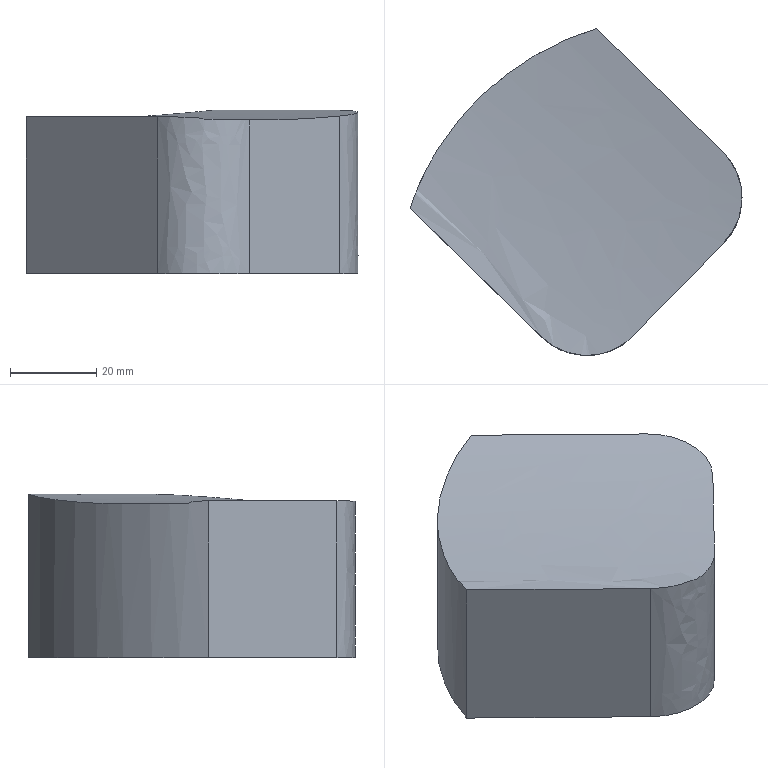Part | NX | features solid 2 | 1 solid | 10 faces | box 76.93 x 75.708 x 37.827 mm | volume 128623 mm3 | spline 6 | plane 2 | cylinder 1 | cone 1 | commonest cylinder face diameters 10 x1
STEP:
#1=CARTESIAN_POINT('',(-596.108,399.175,9.827));
#2=VERTEX_POINT('',#1);
#3=CARTESIAN_POINT('',(-566.89,370.687,9.827));
#4=VERTEX_POINT('',#3);
#5=CARTESIAN_POINT('',(-566.89,370.687,9.827));
#6=CARTESIAN_POINT('',(-576.63,380.183,9.827));
#7=CARTESIAN_POINT('',(-586.369,389.679,9.827));
#8=CARTESIAN_POINT('',(-596.108,399.175,9.827));
#9=B_SPLINE_CURVE_WITH_KNOTS('',3,(#5,#6,#7,#8),.UNSPECIFIED.,.F.,.F.,(4,4),(0.04669,0.0875),.UNSPECIFIED.);
#10=EDGE_CURVE('',#2,#4,#9,.F.);
#11=ORIENTED_EDGE('',*,*,#10,.T.);
#12=CARTESIAN_POINT('',(-566.89,370.687,-28.));
#13=VERTEX_POINT('',#12);
#14=CARTESIAN_POINT('',(-566.89,370.687,9.827));
#15=CARTESIAN_POINT('',(-566.89,370.687,-2.782));
#16=CARTESIAN_POINT('',(-566.89,370.687,-15.391));
#17=CARTESIAN_POINT('',(-566.89,370.687,-28.));
#18=B_SPLINE_CURVE_WITH_KNOTS('',3,(#14,#15,#16,#17),.UNSPECIFIED.,.F.,.F.,(4,4),(0.,0.03783),.UNSPECIFIED.);
#19=EDGE_CURVE('',#4,#13,#18,.T.);
#20=ORIENTED_EDGE('',*,*,#19,.T.);
#21=CARTESIAN_POINT('',(-596.108,399.175,-28.));
#22=VERTEX_POINT('',#21);
#23=CARTESIAN_POINT('',(-596.108,399.175,-28.));
#24=CARTESIAN_POINT('',(-586.369,389.679,-28.));
#25=CARTESIAN_POINT('',(-576.63,380.183,-28.));
#26=CARTESIAN_POINT('',(-566.89,370.687,-28.));
#27=B_SPLINE_CURVE_WITH_KNOTS('',3,(#23,#24,#25,#26),.UNSPECIFIED.,.F.,.F.,(4,4),(0.,1.),.UNSPECIFIED.);
#28=EDGE_CURVE('',#22,#13,#27,.T.);
#29=ORIENTED_EDGE('',*,*,#28,.F.);
#30=CARTESIAN_POINT('',(-596.108,399.175,-28.));
#31=CARTESIAN_POINT('',(-596.108,399.175,-15.391));
#32=CARTESIAN_POINT('',(-596.108,399.175,-2.782));
#33=CARTESIAN_POINT('',(-596.108,399.175,9.827));
#34=B_SPLINE_CURVE_WITH_KNOTS('',3,(#30,#31,#32,#33),.UNSPECIFIED.,.F.,.F.,(4,4),(0.164,0.2018),.UNSPECIFIED.);
#35=EDGE_CURVE('',#22,#2,#34,.T.);
#36=ORIENTED_EDGE('',*,*,#35,.T.);
#37=EDGE_LOOP('',(#11,#20,#29,#36));
#38=FACE_BOUND('',#37,.T.);
#39=CARTESIAN_POINT('',(-566.89,370.687,9.827));
#40=CARTESIAN_POINT('',(-576.63,380.183,9.827));
#41=CARTESIAN_POINT('',(-586.369,389.679,9.827));
#42=CARTESIAN_POINT('',(-596.108,399.175,9.827));
#43=CARTESIAN_POINT('',(-566.89,370.687,-2.782));
#44=CARTESIAN_POINT('',(-576.63,380.183,-2.782));
#45=CARTESIAN_POINT('',(-586.369,389.679,-2.782));
#46=CARTESIAN_POINT('',(-596.108,399.175,-2.782));
#47=CARTESIAN_POINT('',(-566.89,370.687,-15.391));
#48=CARTESIAN_POINT('',(-576.63,380.183,-15.391));
#49=CARTESIAN_POINT('',(-586.369,389.679,-15.391));
#50=CARTESIAN_POINT('',(-596.108,399.175,-15.391));
#51=CARTESIAN_POINT('',(-566.89,370.687,-28.));
#52=CARTESIAN_POINT('',(-576.63,380.183,-28.));
#53=CARTESIAN_POINT('',(-586.369,389.679,-28.));
#54=CARTESIAN_POINT('',(-596.108,399.175,-28.));
#55=B_SPLINE_SURFACE_WITH_KNOTS('',3,3,((#39,#40,#41,#42),(#43,#44,#45,#46),(#47,#48,#49,#50),(#51,#52,#53,#54)),.UNSPECIFIED.,.F.,.F.,.F.,(4,4),(4,4),(0.2675,0.6667),(0.57,0.7724),.UNSPECIFIED.);
#56=ADVANCED_FACE('',(#38),#55,.T.);
#57=CARTESIAN_POINT('',(-639.292,357.48,-28.));
#58=VERTEX_POINT('',#57);
#59=CARTESIAN_POINT('',(-608.776,327.727,-28.));
#60=VERTEX_POINT('',#59);
#61=CARTESIAN_POINT('',(-608.776,327.727,-28.));
#62=CARTESIAN_POINT('',(-618.948,337.645,-28.));
#63=CARTESIAN_POINT('',(-629.12,347.562,-28.));
#64=CARTESIAN_POINT('',(-639.292,357.48,-28.));
#65=B_SPLINE_CURVE_WITH_KNOTS('',3,(#61,#62,#63,#64),.UNSPECIFIED.,.F.,.F.,(4,4),(0.,1.),.UNSPECIFIED.);
#66=EDGE_CURVE('',#58,#60,#65,.F.);
#67=ORIENTED_EDGE('',*,*,#66,.T.);
#68=CARTESIAN_POINT('',(-608.776,327.727,8.344));
#69=VERTEX_POINT('',#68);
#70=CARTESIAN_POINT('',(-608.776,327.727,-28.));
#71=CARTESIAN_POINT('',(-608.776,327.727,-15.885));
#72=CARTESIAN_POINT('',(-608.776,327.727,-3.77));
#73=CARTESIAN_POINT('',(-608.776,327.727,8.344));
#74=B_SPLINE_CURVE_WITH_KNOTS('',3,(#70,#71,#72,#73),.UNSPECIFIED.,.F.,.F.,(4,4),(0.,0.03634),.UNSPECIFIED.);
#75=EDGE_CURVE('',#60,#69,#74,.T.);
#76=ORIENTED_EDGE('',*,*,#75,.T.);
#77=CARTESIAN_POINT('',(-639.292,357.48,8.344));
#78=VERTEX_POINT('',#77);
#79=CARTESIAN_POINT('',(-639.292,357.48,8.344));
#80=CARTESIAN_POINT('',(-629.12,347.562,8.344));
#81=CARTESIAN_POINT('',(-618.948,337.645,8.344));
#82=CARTESIAN_POINT('',(-608.776,327.727,8.344));
#83=B_SPLINE_CURVE_WITH_KNOTS('',3,(#79,#80,#81,#82),.UNSPECIFIED.,.F.,.F.,(4,4),(0.3802,0.4229),.UNSPECIFIED.);
#84=EDGE_CURVE('',#78,#69,#83,.T.);
#85=ORIENTED_EDGE('',*,*,#84,.F.);
#86=CARTESIAN_POINT('',(-639.292,357.48,-28.));
#87=CARTESIAN_POINT('',(-639.292,357.48,-15.885));
#88=CARTESIAN_POINT('',(-639.292,357.48,-3.77));
#89=CARTESIAN_POINT('',(-639.292,357.48,8.344));
#90=B_SPLINE_CURVE_WITH_KNOTS('',3,(#86,#87,#88,#89),.UNSPECIFIED.,.F.,.F.,(4,4),(0.1647,0.2011),.UNSPECIFIED.);
#91=EDGE_CURVE('',#58,#78,#90,.T.);
#92=ORIENTED_EDGE('',*,*,#91,.F.);
#93=EDGE_LOOP('',(#67,#76,#85,#92));
#94=FACE_BOUND('',#93,.T.);
#95=CARTESIAN_POINT('',(-608.776,327.727,-28.));
#96=CARTESIAN_POINT('',(-608.776,327.727,-15.885));
#97=CARTESIAN_POINT('',(-608.776,327.727,-3.77));
#98=CARTESIAN_POINT('',(-608.776,327.727,8.344));
#99=CARTESIAN_POINT('',(-618.948,337.645,-28.));
#100=CARTESIAN_POINT('',(-618.948,337.645,-15.885));
#101=CARTESIAN_POINT('',(-618.948,337.645,-3.77));
#102=CARTESIAN_POINT('',(-618.948,337.645,8.344));
#103=CARTESIAN_POINT('',(-629.12,347.562,-28.));
#104=CARTESIAN_POINT('',(-629.12,347.562,-15.885));
#105=CARTESIAN_POINT('',(-629.12,347.562,-3.77));
#106=CARTESIAN_POINT('',(-629.12,347.562,8.344));
#107=CARTESIAN_POINT('',(-639.292,357.48,-28.));
#108=CARTESIAN_POINT('',(-639.292,357.48,-15.885));
#109=CARTESIAN_POINT('',(-639.292,357.48,-3.77));
#110=CARTESIAN_POINT('',(-639.292,357.48,8.344));
#111=B_SPLINE_SURFACE_WITH_KNOTS('',3,3,((#95,#96,#97,#98),(#99,#100,#101,#102),(#103,#104,#105,#106),(#107,#108,#109,#110)),.UNSPECIFIED.,.F.,.F.,.F.,(4,4),(4,4),(0.5587,0.76),(0.3333,0.6894),.UNSPECIFIED.);
#112=ADVANCED_FACE('',(#94),#111,.F.);
#113=ORIENTED_EDGE('',*,*,#84,.T.);
#114=CARTESIAN_POINT('',(-587.565,327.996,7.602));
#115=VERTEX_POINT('',#114);
#116=CARTESIAN_POINT('',(-608.776,327.727,8.344));
#117=CARTESIAN_POINT('',(-608.068,327.037,8.344));
#118=CARTESIAN_POINT('',(-606.545,325.819,8.337));
#119=CARTESIAN_POINT('',(-604.346,324.676,8.3));
#120=CARTESIAN_POINT('',(-602.494,324.04,8.277));
#121=CARTESIAN_POINT('',(-601.076,323.7,8.186));
#122=CARTESIAN_POINT('',(-599.594,323.499,8.343));
#123=CARTESIAN_POINT('',(-598.174,323.445,7.686));
#124=CARTESIAN_POINT('',(-596.694,323.529,7.792));
#125=CARTESIAN_POINT('',(-595.235,323.76,7.739));
#126=CARTESIAN_POINT('',(-593.792,324.137,7.712));
#127=CARTESIAN_POINT('',(-591.034,325.156,7.65));
#128=CARTESIAN_POINT('',(-588.952,326.573,7.616));
#129=CARTESIAN_POINT('',(-587.565,327.996,7.602));
#130=B_SPLINE_CURVE_WITH_KNOTS('',3,(#116,#117,#118,#119,#120,#121,#122,#123,#124,#125,#126,#127,#128,#129),.UNSPECIFIED.,.F.,.F.,(4,1,1,1,1,1,1,1,1,1,1,4),(0.,0.002926,0.005852,0.007315,0.008778,0.01024,0.0117,0.01317,0.01463,0.01609,0.01756,0.02341),.UNSPECIFIED.);
#131=EDGE_CURVE('',#69,#115,#130,.T.);
#132=ORIENTED_EDGE('',*,*,#131,.T.);
#133=CARTESIAN_POINT('',(-566.622,349.476,8.518));
#134=VERTEX_POINT('',#133);
#135=CARTESIAN_POINT('',(-566.622,349.476,8.518));
#136=CARTESIAN_POINT('',(-573.593,342.326,7.847));
#137=CARTESIAN_POINT('',(-580.587,335.153,7.534));
#138=CARTESIAN_POINT('',(-587.565,327.996,7.602));
#139=B_SPLINE_CURVE_WITH_KNOTS('',3,(#135,#136,#137,#138),.UNSPECIFIED.,.F.,.F.,(4,4),(0.1635,0.1938),.UNSPECIFIED.);
#140=EDGE_CURVE('',#134,#115,#139,.T.);
#141=ORIENTED_EDGE('',*,*,#140,.F.);
#142=CARTESIAN_POINT('',(-566.622,349.476,8.518));
#143=CARTESIAN_POINT('',(-565.24,350.893,8.651));
#144=CARTESIAN_POINT('',(-563.079,354.228,8.942));
#145=CARTESIAN_POINT('',(-561.596,362.099,9.545));
#146=CARTESIAN_POINT('',(-564.049,367.916,9.827));
#147=CARTESIAN_POINT('',(-566.89,370.687,9.827));
#148=B_SPLINE_CURVE_WITH_KNOTS('',3,(#142,#143,#144,#145,#146,#147),.UNSPECIFIED.,.F.,.F.,(4,1,1,4),(0.,0.005869,0.01174,0.02347),.UNSPECIFIED.);
#149=EDGE_CURVE('',#134,#4,#148,.T.);
#150=ORIENTED_EDGE('',*,*,#149,.T.);
#151=ORIENTED_EDGE('',*,*,#10,.F.);
#152=CARTESIAN_POINT('',(-639.292,357.48,8.344));
#153=CARTESIAN_POINT('',(-639.092,358.095,8.318));
#154=CARTESIAN_POINT('',(-638.778,359.015,8.297));
#155=CARTESIAN_POINT('',(-638.33,360.228,8.196));
#156=CARTESIAN_POINT('',(-638.033,360.994,8.289));
#157=CARTESIAN_POINT('',(-637.799,361.576,7.931));
#158=CARTESIAN_POINT('',(-637.556,362.168,7.731));
#159=CARTESIAN_POINT('',(-637.235,362.924,7.781));
#160=CARTESIAN_POINT('',(-636.837,363.821,7.751));
#161=CARTESIAN_POINT('',(-636.285,365.014,7.722));
#162=CARTESIAN_POINT('',(-635.563,366.482,7.684));
#163=CARTESIAN_POINT('',(-634.338,368.784,7.637));
#164=CARTESIAN_POINT('',(-632.014,372.69,7.583));
#165=CARTESIAN_POINT('',(-628.209,377.922,7.593));
#166=CARTESIAN_POINT('',(-621.036,385.625,7.825));
#167=CARTESIAN_POINT('',(-612.759,391.866,8.343));
#168=CARTESIAN_POINT('',(-603.408,396.636,9.12));
#169=CARTESIAN_POINT('',(-598.574,398.42,9.579));
#170=CARTESIAN_POINT('',(-596.108,399.175,9.827));
#171=B_SPLINE_CURVE_WITH_KNOTS('',3,(#152,#153,#154,#155,#156,#157,#158,#159,#160,#161,#162,#163,#164,#165,#166,#167,#168,#169,#170),.UNSPECIFIED.,.F.,.F.,(4,1,1,1,1,1,1,1,1,1,1,1,1,1,1,1,4),(0.0326,0.03455,0.03553,0.03651,0.037,0.03748,0.03846,0.03944,0.04041,0.04237,0.04432,0.04823,0.05604,0.06386,0.07949,0.0873,0.09512),.UNSPECIFIED.);
#172=EDGE_CURVE('',#78,#2,#171,.T.);
#173=ORIENTED_EDGE('',*,*,#172,.F.);
#174=EDGE_LOOP('',(#113,#132,#141,#150,#151,#173));
#175=FACE_BOUND('',#174,.T.);
#176=CARTESIAN_POINT('',(-593.046,312.39,8.344));
#177=CARTESIAN_POINT('',(-639.573,357.754,8.344));
#178=CARTESIAN_POINT('',(-592.844,313.009,8.317));
#179=CARTESIAN_POINT('',(-639.372,358.373,8.317));
#180=CARTESIAN_POINT('',(-592.526,313.934,8.289));
#181=CARTESIAN_POINT('',(-639.054,359.299,8.289));
#182=CARTESIAN_POINT('',(-592.076,315.149,8.208));
#183=CARTESIAN_POINT('',(-638.604,360.513,8.208));
#184=CARTESIAN_POINT('',(-591.716,316.074,8.264));
#185=CARTESIAN_POINT('',(-638.243,361.439,8.264));
#186=CARTESIAN_POINT('',(-591.391,316.873,7.698));
#187=CARTESIAN_POINT('',(-637.918,362.237,7.698));
#188=CARTESIAN_POINT('',(-590.999,317.799,7.788));
#189=CARTESIAN_POINT('',(-637.526,363.163,7.788));
#190=CARTESIAN_POINT('',(-590.606,318.685,7.75));
#191=CARTESIAN_POINT('',(-637.133,364.049,7.75));
#192=CARTESIAN_POINT('',(-590.058,319.87,7.725));
#193=CARTESIAN_POINT('',(-636.586,365.234,7.725));
#194=CARTESIAN_POINT('',(-589.342,321.331,7.685));
#195=CARTESIAN_POINT('',(-635.869,366.695,7.685));
#196=CARTESIAN_POINT('',(-588.122,323.634,7.639));
#197=CARTESIAN_POINT('',(-634.65,368.999,7.639));
#198=CARTESIAN_POINT('',(-585.804,327.564,7.583));
#199=CARTESIAN_POINT('',(-632.332,372.928,7.583));
#200=CARTESIAN_POINT('',(-581.987,332.856,7.594));
#201=CARTESIAN_POINT('',(-628.514,378.22,7.594));
#202=CARTESIAN_POINT('',(-574.891,340.502,7.822));
#203=CARTESIAN_POINT('',(-621.418,385.867,7.822));
#204=CARTESIAN_POINT('',(-564.414,348.385,8.475));
#205=CARTESIAN_POINT('',(-610.941,393.75,8.475));
#206=CARTESIAN_POINT('',(-554.827,352.572,9.328));
#207=CARTESIAN_POINT('',(-601.355,397.936,9.328));
#208=CARTESIAN_POINT('',(-549.867,354.089,9.827));
#209=CARTESIAN_POINT('',(-596.394,399.453,9.827));
#210=B_SPLINE_SURFACE_WITH_KNOTS('',3,1,((#176,#177),(#178,#179),(#180,#181),(#182,#183),(#184,#185),(#186,#187),(#188,#189),(#190,#191),(#192,#193),(#194,#195),(#196,#197),(#198,#199),(#200,#201),(#202,#203),(#204,#205),(#206,#207),(#208,#209)),.SURF_OF_LINEAR_EXTRUSION.,.F.,.F.,.F.,(4,1,1,1,1,1,1,1,1,1,1,1,1,1,4),(2,2),(0.3494,0.3597,0.3649,0.3701,0.3752,0.3804,0.3856,0.3908,0.4011,0.4114,0.4321,0.4735,0.5149,0.5976,0.6803),(0.,1.),.UNSPECIFIED.);
#211=ADVANCED_FACE('',(#175),#210,.T.);
#212=CARTESIAN_POINT('',(-593.573,359.679,-28.));
#213=VERTEX_POINT('',#212);
#214=CARTESIAN_POINT('',(-598.573,359.679,-28.));
#215=DIRECTION('',(0.,0.,1.));
#216=DIRECTION('',(1.,0.,0.));
#217=AXIS2_PLACEMENT_3D('',#214,#215,#216);
#218=CIRCLE('',#217,5.);
#219=EDGE_CURVE('',#213,#213,#218,.F.);
#220=ORIENTED_EDGE('',*,*,#219,.F.);
#221=EDGE_LOOP('',(#220));
#222=FACE_BOUND('',#221,.T.);
#223=CARTESIAN_POINT('',(-587.565,327.996,-28.));
#224=VERTEX_POINT('',#223);
#225=CARTESIAN_POINT('',(-566.622,349.476,-28.));
#226=VERTEX_POINT('',#225);
#227=CARTESIAN_POINT('',(-597.903,317.393,-28.));
#228=DIRECTION('',(-0.6981,-0.716,0.));
#229=VECTOR('',#228,1000.);
#230=LINE('',#227,#229);
#231=EDGE_CURVE('',#224,#226,#230,.F.);
#232=ORIENTED_EDGE('',*,*,#231,.F.);
#233=CARTESIAN_POINT('',(-598.305,338.467,-28.));
#234=DIRECTION('',(0.,0.,1.));
#235=DIRECTION('',(1.,0.,0.));
#236=AXIS2_PLACEMENT_3D('',#233,#234,#235);
#237=CIRCLE('',#236,15.);
#238=EDGE_CURVE('',#224,#60,#237,.F.);
#239=ORIENTED_EDGE('',*,*,#238,.T.);
#240=ORIENTED_EDGE('',*,*,#66,.F.);
#241=CARTESIAN_POINT('',(-639.292,357.48,-28.));
#242=CARTESIAN_POINT('',(-638.489,359.955,-28.));
#243=CARTESIAN_POINT('',(-636.589,364.763,-28.));
#244=CARTESIAN_POINT('',(-632.75,371.685,-28.));
#245=CARTESIAN_POINT('',(-628.221,377.908,-28.));
#246=CARTESIAN_POINT('',(-621.062,385.605,-28.));
#247=CARTESIAN_POINT('',(-610.608,393.47,-28.));
#248=CARTESIAN_POINT('',(-601.102,397.646,-28.));
#249=CARTESIAN_POINT('',(-596.108,399.175,-28.));
#250=B_SPLINE_CURVE_WITH_KNOTS('',3,(#241,#242,#243,#244,#245,#246,#247,#248,#249),.UNSPECIFIED.,.F.,.F.,(4,1,1,1,1,1,4),(0.,0.125,0.25,0.375,0.5,0.75,1.),.UNSPECIFIED.);
#251=EDGE_CURVE('',#22,#58,#250,.F.);
#252=ORIENTED_EDGE('',*,*,#251,.F.);
#253=ORIENTED_EDGE('',*,*,#28,.T.);
#254=CARTESIAN_POINT('',(-577.362,359.947,-28.));
#255=DIRECTION('',(0.,0.,1.));
#256=DIRECTION('',(1.,0.,0.));
#257=AXIS2_PLACEMENT_3D('',#254,#255,#256);
#258=CIRCLE('',#257,15.);
#259=EDGE_CURVE('',#13,#226,#258,.F.);
#260=ORIENTED_EDGE('',*,*,#259,.T.);
#261=EDGE_LOOP('',(#232,#239,#240,#252,#253,#260));
#262=FACE_BOUND('',#261,.T.);
#263=CARTESIAN_POINT('',(-592.5,65.,-28.));
#264=DIRECTION('',(0.,0.,1.));
#265=DIRECTION('',(1.,0.,0.));
#266=AXIS2_PLACEMENT_3D('',#263,#264,#265);
#267=PLANE('',#266);
#268=ADVANCED_FACE('',(#222,#262),#267,.F.);
#269=ORIENTED_EDGE('',*,*,#35,.F.);
#270=ORIENTED_EDGE('',*,*,#251,.T.);
#271=ORIENTED_EDGE('',*,*,#91,.T.);
#272=ORIENTED_EDGE('',*,*,#172,.T.);
#273=EDGE_LOOP('',(#269,#270,#271,#272));
#274=FACE_BOUND('',#273,.T.);
#275=CARTESIAN_POINT('',(-596.108,399.175,-28.));
#276=CARTESIAN_POINT('',(-596.108,399.175,10.054));
#277=CARTESIAN_POINT('',(-606.018,396.141,-28.));
#278=CARTESIAN_POINT('',(-606.018,396.141,10.054));
#279=CARTESIAN_POINT('',(-624.458,385.365,-28.));
#280=CARTESIAN_POINT('',(-624.458,385.365,10.054));
#281=CARTESIAN_POINT('',(-636.086,367.37,-28.));
#282=CARTESIAN_POINT('',(-636.086,367.37,10.054));
#283=CARTESIAN_POINT('',(-639.292,357.48,-28.));
#284=CARTESIAN_POINT('',(-639.292,357.48,10.054));
#285=B_SPLINE_SURFACE_WITH_KNOTS('',3,1,((#275,#276),(#277,#278),(#279,#280),(#281,#282),(#283,#284)),.SURF_OF_LINEAR_EXTRUSION.,.F.,.F.,.F.,(4,1,4),(2,2),(0.3233,0.3364,0.3495),(0.,1.),.UNSPECIFIED.);
#286=ADVANCED_FACE('',(#274),#285,.T.);
#287=ORIENTED_EDGE('',*,*,#140,.T.);
#288=CARTESIAN_POINT('',(-587.565,327.996,7.602));
#289=CARTESIAN_POINT('',(-587.565,327.996,-4.265));
#290=CARTESIAN_POINT('',(-587.565,327.996,-16.133));
#291=CARTESIAN_POINT('',(-587.565,327.996,-28.));
#292=B_SPLINE_CURVE_WITH_KNOTS('',3,(#288,#289,#290,#291),.UNSPECIFIED.,.F.,.F.,(4,4),(0.,0.0356),.UNSPECIFIED.);
#293=EDGE_CURVE('',#115,#224,#292,.T.);
#294=ORIENTED_EDGE('',*,*,#293,.T.);
#295=ORIENTED_EDGE('',*,*,#231,.T.);
#296=CARTESIAN_POINT('',(-566.622,349.476,-28.));
#297=CARTESIAN_POINT('',(-566.622,349.476,-15.827));
#298=CARTESIAN_POINT('',(-566.622,349.476,-3.655));
#299=CARTESIAN_POINT('',(-566.622,349.476,8.518));
#300=B_SPLINE_CURVE_WITH_KNOTS('',3,(#296,#297,#298,#299),.UNSPECIFIED.,.F.,.F.,(4,4),(0.,0.03652),.UNSPECIFIED.);
#301=EDGE_CURVE('',#226,#134,#300,.T.);
#302=ORIENTED_EDGE('',*,*,#301,.T.);
#303=EDGE_LOOP('',(#287,#294,#295,#302));
#304=FACE_BOUND('',#303,.T.);
#305=CARTESIAN_POINT('',(-597.903,317.393,-18.));
#306=DIRECTION('',(0.716,-0.6981,0.));
#307=DIRECTION('',(0.6981,0.716,0.));
#308=AXIS2_PLACEMENT_3D('',#305,#306,#307);
#309=PLANE('',#308);
#310=ADVANCED_FACE('',(#304),#309,.T.);
#311=ORIENTED_EDGE('',*,*,#219,.T.);
#312=EDGE_LOOP('',(#311));
#313=FACE_BOUND('',#312,.T.);
#314=CARTESIAN_POINT('',(-593.573,359.679,-7.5));
#315=VERTEX_POINT('',#314);
#316=CARTESIAN_POINT('',(-598.573,359.679,-7.5));
#317=DIRECTION('',(0.,0.,1.));
#318=DIRECTION('',(1.,0.,0.));
#319=AXIS2_PLACEMENT_3D('',#316,#317,#318);
#320=CIRCLE('',#319,5.);
#321=EDGE_CURVE('',#315,#315,#320,.T.);
#322=ORIENTED_EDGE('',*,*,#321,.T.);
#323=EDGE_LOOP('',(#322));
#324=FACE_BOUND('',#323,.T.);
#325=CARTESIAN_POINT('',(-598.573,359.679,-52.5));
#326=DIRECTION('',(0.,0.,1.));
#327=DIRECTION('',(1.,0.,0.));
#328=AXIS2_PLACEMENT_3D('',#325,#326,#327);
#329=CYLINDRICAL_SURFACE('',#328,5.);
#330=ADVANCED_FACE('',(#313,#324),#329,.F.);
#331=ORIENTED_EDGE('',*,*,#238,.F.);
#332=ORIENTED_EDGE('',*,*,#293,.F.);
#333=ORIENTED_EDGE('',*,*,#131,.F.);
#334=ORIENTED_EDGE('',*,*,#75,.F.);
#335=EDGE_LOOP('',(#331,#332,#333,#334));
#336=FACE_BOUND('',#335,.T.);
#337=CARTESIAN_POINT('',(-587.565,327.996,-28.));
#338=CARTESIAN_POINT('',(-598.036,317.256,-28.));
#339=CARTESIAN_POINT('',(-608.776,327.727,-28.));
#340=CARTESIAN_POINT('',(-587.565,327.996,-15.81));
#341=CARTESIAN_POINT('',(-598.036,317.256,-15.81));
#342=CARTESIAN_POINT('',(-608.776,327.727,-15.81));
#343=CARTESIAN_POINT('',(-587.565,327.996,-3.621));
#344=CARTESIAN_POINT('',(-598.036,317.256,-3.621));
#345=CARTESIAN_POINT('',(-608.776,327.727,-3.621));
#346=CARTESIAN_POINT('',(-587.565,327.996,8.569));
#347=CARTESIAN_POINT('',(-598.036,317.256,8.569));
#348=CARTESIAN_POINT('',(-608.776,327.727,8.569));
#349=(BOUNDED_SURFACE()B_SPLINE_SURFACE(3,2,((#337,#338,#339),(#340,#341,#342),(#343,#344,#345),(#346,#347,#348)),.UNSPECIFIED.,.F.,.F.,.F.)B_SPLINE_SURFACE_WITH_KNOTS((4,4),(3,3),(0.03287,0.06944),(0.,1.),.PIECEWISE_BEZIER_KNOTS.)GEOMETRIC_REPRESENTATION_ITEM()RATIONAL_B_SPLINE_SURFACE(((1.,0.7071,1.),(1.,0.7071,1.),(1.,0.7071,1.),(1.,0.7071,1.)))REPRESENTATION_ITEM('')SURFACE());
#350=ADVANCED_FACE('',(#336),#349,.T.);
#351=ORIENTED_EDGE('',*,*,#149,.F.);
#352=ORIENTED_EDGE('',*,*,#301,.F.);
#353=ORIENTED_EDGE('',*,*,#259,.F.);
#354=ORIENTED_EDGE('',*,*,#19,.F.);
#355=EDGE_LOOP('',(#351,#352,#353,#354));
#356=FACE_BOUND('',#355,.T.);
#357=CARTESIAN_POINT('',(-566.622,349.476,10.054));
#358=CARTESIAN_POINT('',(-556.15,360.216,10.054));
#359=CARTESIAN_POINT('',(-566.89,370.687,10.054));
#360=CARTESIAN_POINT('',(-566.622,349.476,-2.631));
#361=CARTESIAN_POINT('',(-556.15,360.216,-2.631));
#362=CARTESIAN_POINT('',(-566.89,370.687,-2.631));
#363=CARTESIAN_POINT('',(-566.622,349.476,-15.315));
#364=CARTESIAN_POINT('',(-556.15,360.216,-15.315));
#365=CARTESIAN_POINT('',(-566.89,370.687,-15.315));
#366=CARTESIAN_POINT('',(-566.622,349.476,-28.));
#367=CARTESIAN_POINT('',(-556.15,360.216,-28.));
#368=CARTESIAN_POINT('',(-566.89,370.687,-28.));
#369=(BOUNDED_SURFACE()B_SPLINE_SURFACE(3,2,((#357,#358,#359),(#360,#361,#362),(#363,#364,#365),(#366,#367,#368)),.UNSPECIFIED.,.F.,.F.,.F.)B_SPLINE_SURFACE_WITH_KNOTS((4,4),(3,3),(0.123,0.1611),(0.,1.),.PIECEWISE_BEZIER_KNOTS.)GEOMETRIC_REPRESENTATION_ITEM()RATIONAL_B_SPLINE_SURFACE(((1.,0.7071,1.),(1.,0.7071,1.),(1.,0.7071,1.),(1.,0.7071,1.)))REPRESENTATION_ITEM('')SURFACE());
#370=ADVANCED_FACE('',(#356),#369,.T.);
#371=ORIENTED_EDGE('',*,*,#321,.F.);
#372=EDGE_LOOP('',(#371));
#373=FACE_BOUND('',#372,.T.);
#374=CARTESIAN_POINT('',(-598.573,359.679,-4.496));
#375=VERTEX_POINT('',#374);
#376=VERTEX_LOOP('',#375);
#377=FACE_BOUND('',#376,.T.);
#378=CARTESIAN_POINT('',(-598.573,359.679,-7.5));
#379=DIRECTION('',(0.,0.,-1.));
#380=DIRECTION('',(-1.,0.,0.));
#381=AXIS2_PLACEMENT_3D('',#378,#379,#380);
#382=CONICAL_SURFACE('',#381,5.,1.03);
#383=ADVANCED_FACE('',(#373,#377),#382,.F.);
#384=CLOSED_SHELL('',(#56,#112,#211,#268,#286,#310,#330,#350,#370,#383));
#385=MANIFOLD_SOLID_BREP('',#384);
#386=(LENGTH_UNIT()NAMED_UNIT(*)SI_UNIT(.MILLI.,.METRE.));
#387=UNCERTAINTY_MEASURE_WITH_UNIT(LENGTH_MEASURE(0.0508),#386,'','');
#388=(NAMED_UNIT(*)PLANE_ANGLE_UNIT()SI_UNIT($,.RADIAN.));
#389=(NAMED_UNIT(*)SI_UNIT($,.STERADIAN.)SOLID_ANGLE_UNIT());
#390=(GEOMETRIC_REPRESENTATION_CONTEXT(3)GLOBAL_UNCERTAINTY_ASSIGNED_CONTEXT((#387))GLOBAL_UNIT_ASSIGNED_CONTEXT((#386,#388,#389))REPRESENTATION_CONTEXT('',''));
#391=ADVANCED_BREP_SHAPE_REPRESENTATION('',(#385),#390);